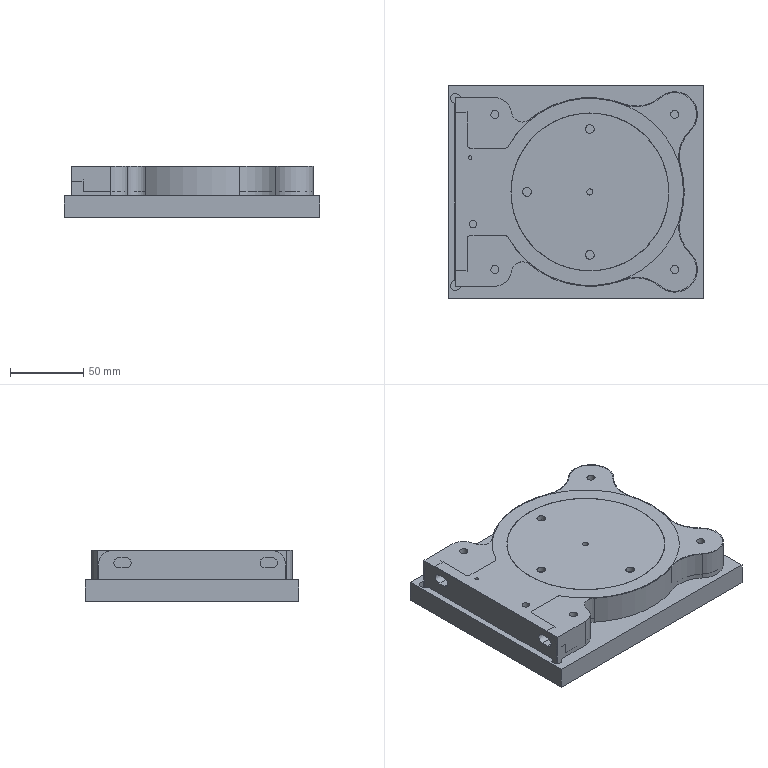NC program | NX | posted with a generic post | part box 175 x 146 x 35 mm
Lines 1 to 998 of 35144:
N10 G17 G21 G94 G90
(正面_COPY , TOOL : D10)
N12 T02 M6
N14 G54
N16 G17 G0 G90 X95.5 Y-68.762 S8000 M3
N18 G43 Z20. H2
N20 Z0.15
N22 G94 G1 X90.5 F2000.
N24 X-90.5
N26 Y-61.524
N28 X90.5
N30 Y-54.286
N32 X-90.5
N34 Y-47.048
N36 X90.5
N38 Y-39.81
N40 X-90.5
N42 Y-32.571
N44 X90.5
N46 Y-25.333
N48 X-90.5
N50 Y-18.095
N52 X90.5
N54 Y-10.857
N56 X-90.5
N58 Y-3.619
N60 X90.5
N62 Y3.619
N64 X-90.5
N66 Y10.857
N68 X90.5
N70 Y18.095
N72 X-90.5
N74 Y25.333
N76 X90.5
N78 Y32.571
N80 X-90.5
N82 Y39.81
N84 X90.5
N86 Y47.048
N88 X-90.5
N90 Y54.286
N92 X90.5
N94 Y61.524
N96 X-90.5
N98 Y68.762
N100 X90.5
N102 X95.5
N104 G0 Z20.
(跟随部件_COPY_2 , TOOL : D10)
N106 G1 X99.568 Y27.523 F15000.
N108 Z-1.4
N110 Z-1.9 F4000.
N112 G3 X92.497 Y27.582 R5.
N114 G2 X92.161 Y27.256 R35.65
N116 G3 X90.983 Y22.936 R4.35
N118 G2 X92.497 Y16.648 R84.65
N120 G3 X98.382 Y12.73 R5.
N122 G1 Z-1.4
N124 Z20. F15000.
N126 Y-12.73
N128 Z-1.4
N130 Z-1.9 F4000.
N132 G3 X92.497 Y-16.648 R5.
N134 G2 X90.983 Y-22.936 R84.65
N136 G3 X92.161 Y-27.256 R4.35
N138 G2 X92.497 Y-27.582 R35.65
N140 G1 Y-40.054
N142 G3 X86.973 Y-32.672 R28.15
N144 G2 X83.764 Y-20.904 R11.85
N146 G3 X83.764 Y20.904 R77.15
N148 G2 X86.973 Y32.672 R11.85
N150 G3 X92.497 Y40.054 R28.15
N152 G2 X99.236 Y42.195 R5.
N154 G1 Z-1.4
N156 Z20. F15000.
N158 X-36.967 Y85.011
N160 Z-1.4
N162 Z-1.9 F4000.
N164 G3 X-36.085 Y77.996 R5.
N166 G2 X-31.749 Y73.92 R31.65
N168 X-23.399 Y77.996 R84.65
N170 G3 X-20.735 Y84.546 R5.
N172 G1 Z-1.4
N174 Z20. F15000.
N176 X56.692 Y84.735
N178 Z-1.4
N180 Z-1.9 F4000.
N182 G2 X54.552 Y77.996 R5.
N184 G3 X49.005 Y74.222 R28.15
N186 G2 X36.997 Y72.084 R11.85
N188 G3 X-33.894 Y63.789 R77.15
N190 X-55.5 Y77.15 R24.15
N192 G1 X-82.502
N194 G3 X-92.497 Y72.543 R13.15
N196 G2 X-99.546 Y71.991 R5.
N198 G1 Z-1.4
N200 Z20. F15000.
N202 X-20.735 Y-84.546
N204 Z-1.4
N206 Z-1.9 F4000.
N208 G3 X-23.399 Y-77.996 R5.
N210 G2 X-31.749 Y-73.92 R84.65
N212 X-36.085 Y-77.996 R31.65
N214 G3 X-36.967 Y-85.011 R5.
N216 G1 Z-1.4
N218 Z20. F15000.
N220 X-99.546 Y-71.991
N222 Z-1.4
N224 Z-1.9 F4000.
N226 G2 X-92.497 Y-72.543 R5.
N228 G3 X-82.5 Y-77.15 R13.15
N230 G1 X-55.5
N232 G3 X-33.894 Y-63.789 R24.15
N234 X36.997 Y-72.084 R77.15
N236 G2 X49.005 Y-74.222 R11.85
N238 G3 X54.552 Y-77.996 R28.15
N240 G2 X56.692 Y-84.735 R5.
N242 G1 Z-1.4
N244 Z20. F15000.
N246 X78.308
N248 Z-1.4
N250 Z-1.9 F4000.
N252 G2 X80.448 Y-77.996 R5.
N254 G3 X92.497 Y-65.946 R28.15
N256 G2 X99.236 Y-63.805 R5.
N258 G1 Z-1.4
N260 Z20. F15000.
N262 Y63.805
N264 Z-1.4
N266 Z-1.9 F4000.
N268 G2 X92.497 Y65.946 R5.
N270 G3 X80.448 Y77.996 R28.15
N272 G1 X76.998 Y71.336
N274 G2 X81.785 Y38.088 R20.65
N276 G3 X76.545 Y18.872 R19.35
N278 G2 X76.545 Y-18.872 R69.65
N280 G3 X81.785 Y-38.088 R19.35
N282 G2 X53.933 Y-68.568 R20.65
N284 G3 X34.324 Y-65.076 R19.35
N286 G2 X-35.131 Y-53.472 R69.65
N288 G3 X-38.97 Y-54.994 R2.35
N290 G2 X-55.5 Y-69.65 R16.65
N292 G1 X-82.5
N294 G2 X-88.15 Y-64. R5.65
N296 G1 Y64.
N298 G2 X-82.5 Y69.65 R5.65
N300 G1 X-55.5
N302 G2 X-38.97 Y54.994 R16.65
N304 G3 X-35.131 Y53.472 R2.35
N306 G2 X34.324 Y65.076 R69.65
N308 G3 X53.933 Y68.568 R19.35
N310 G2 X76.998 Y71.336 R20.65
N312 G3 X83.738 Y73.476 R5.
N314 G1 Z-1.4
N316 Z20. F15000.
N318 X99.568 Y27.523
N320 Z-2.9
N322 Z-3.4 F4000.
N324 G3 X92.497 Y27.582 R5.
N326 G2 X92.161 Y27.256 R35.65
N328 G3 X90.983 Y22.936 R4.35
N330 G2 X92.497 Y16.648 R84.65
N332 G3 X98.383 Y12.728 R5.
N334 G1 Z-2.9
N336 Z20. F15000.
N338 Y-12.728
N340 Z-2.9
N342 Z-3.4 F4000.
N344 G3 X92.497 Y-16.648 R5.
N346 G2 X90.983 Y-22.936 R84.65
N348 G3 X92.161 Y-27.256 R4.35
N350 G2 X92.497 Y-27.582 R35.65
N352 G1 Y-40.055
N354 G3 X86.973 Y-32.672 R28.15
N356 G2 X83.764 Y-20.904 R11.85
N358 G3 X83.764 Y20.904 R77.15
N360 G2 X86.973 Y32.672 R11.85
N362 G3 X92.497 Y40.055 R28.15
N364 G2 X99.236 Y42.195 R5.
N366 G1 Z-2.9
N368 Z20. F15000.
N370 X-36.967 Y85.012
N372 Z-2.9
N374 Z-3.4 F4000.
N376 G3 X-36.085 Y77.996 R5.
N378 G2 X-31.749 Y73.92 R31.65
N380 X-23.398 Y77.996 R84.65
N382 G3 X-20.734 Y84.546 R5.
N384 G1 Z-2.9
N386 Z20. F15000.
N388 X56.693 Y84.735
N390 Z-2.9
N392 Z-3.4 F4000.
N394 G2 X54.553 Y77.996 R5.
N396 G3 X49.005 Y74.222 R28.15
N398 G2 X36.997 Y72.084 R11.85
N400 G3 X-33.894 Y63.789 R77.15
N402 X-55.5 Y77.15 R24.15
N404 G1 X-82.502
N406 G3 X-92.497 Y72.543 R13.15
N408 G2 X-99.546 Y71.99 R5.
N410 G1 Z-2.9
N412 Z20. F15000.
N414 X-20.734 Y-84.546
N416 Z-2.9
N418 Z-3.4 F4000.
N420 G3 X-23.398 Y-77.996 R5.
N422 G2 X-31.749 Y-73.92 R84.65
N424 X-36.085 Y-77.996 R31.65
N426 G3 X-36.967 Y-85.012 R5.
N428 G1 Z-2.9
N430 Z20. F15000.
N432 X-99.546 Y-71.99
N434 Z-2.9
N436 Z-3.4 F4000.
N438 G2 X-92.497 Y-72.543 R5.
N440 G3 X-82.5 Y-77.15 R13.15
N442 G1 X-55.5
N444 G3 X-33.894 Y-63.789 R24.15
N446 X36.997 Y-72.084 R77.15
N448 G2 X49.005 Y-74.222 R11.85
N450 G3 X54.553 Y-77.996 R28.15
N452 G2 X56.693 Y-84.735 R5.
N454 G1 Z-2.9
N456 Z20. F15000.
N458 X78.307
N460 Z-2.9
N462 Z-3.4 F4000.
N464 G2 X80.447 Y-77.996 R5.
N466 G3 X92.497 Y-65.945 R28.15
N468 G2 X99.236 Y-63.805 R5.
N470 G1 Z-2.9
N472 Z20. F15000.
N474 Y63.805
N476 Z-2.9
N478 Z-3.4 F4000.
N480 G2 X92.497 Y65.945 R5.
N482 G3 X80.447 Y77.996 R28.15
N484 G1 X76.998 Y71.336
N486 G2 X81.785 Y38.088 R20.65
N488 G3 X76.545 Y18.872 R19.35
N490 G2 X76.545 Y-18.872 R69.65
N492 G3 X81.785 Y-38.088 R19.35
N494 G2 X53.933 Y-68.568 R20.65
N496 G3 X34.324 Y-65.076 R19.35
N498 G2 X-35.131 Y-53.472 R69.65
N500 G3 X-38.97 Y-54.994 R2.35
N502 G2 X-55.5 Y-69.65 R16.65
N504 G1 X-82.5
N506 G2 X-88.15 Y-64. R5.65
N508 G1 Y64.
N510 G2 X-82.5 Y69.65 R5.65
N512 G1 X-55.5
N514 G2 X-38.97 Y54.994 R16.65
N516 G3 X-35.131 Y53.472 R2.35
N518 G2 X34.324 Y65.076 R69.65
N520 G3 X53.933 Y68.568 R19.35
N522 G2 X76.998 Y71.336 R20.65
N524 G3 X83.737 Y73.476 R5.
N526 G1 Z-2.9
N528 Z20. F15000.
N530 X99.568 Y27.523
N532 Z-4.65
N534 Z-5.15 F4000.
N536 G3 X92.497 Y27.582 R5.
N538 G2 X92.161 Y27.256 R35.65
N540 G3 X90.983 Y22.936 R4.35
N542 G2 X92.497 Y16.646 R84.65
N544 G3 X98.383 Y12.727 R5.
N546 G1 Z-4.65
N548 Z20. F15000.
N550 Y-12.727
N552 Z-4.65
N554 Z-5.15 F4000.
N556 G3 X92.497 Y-16.646 R5.
N558 G2 X90.983 Y-22.936 R84.65
N560 G3 X92.161 Y-27.256 R4.35
N562 G2 X92.497 Y-27.582 R35.65
N564 G1 Y-40.055
N566 G3 X86.973 Y-32.672 R28.15
N568 G2 X83.764 Y-20.904 R11.85
N570 G3 X83.764 Y20.904 R77.15
N572 G2 X86.973 Y32.672 R11.85
N574 G3 X92.497 Y40.055 R28.15
N576 G2 X99.236 Y42.196 R5.
N578 G1 Z-4.65
N580 Z20. F15000.
N582 X-36.967 Y85.012
N584 Z-4.65
N586 Z-5.15 F4000.
N588 G3 X-36.086 Y77.996 R5.
N590 G2 X-31.749 Y73.92 R31.65
N592 X-23.397 Y77.996 R84.65
N594 G3 X-20.734 Y84.546 R5.
N596 G1 Z-4.65
N598 Z20. F15000.
N600 X56.693 Y84.735
N602 Z-4.65
N604 Z-5.15 F4000.
N606 G2 X54.553 Y77.996 R5.
N608 G3 X49.005 Y74.222 R28.15
N610 G2 X36.997 Y72.084 R11.85
N612 G3 X-33.894 Y63.789 R77.15
N614 X-55.5 Y77.15 R24.15
N616 G1 X-82.502
N618 G3 X-92.497 Y72.543 R13.15
N620 G2 X-99.547 Y71.99 R5.
N622 G1 Z-4.65
N624 Z20. F15000.
N626 X-20.734 Y-84.546
N628 Z-4.65
N630 Z-5.15 F4000.
N632 G3 X-23.397 Y-77.996 R5.
N634 G2 X-31.749 Y-73.92 R84.65
N636 X-36.086 Y-77.996 R31.65
N638 G3 X-36.967 Y-85.012 R5.
N640 G1 Z-4.65
N642 Z20. F15000.
N644 X-99.547 Y-71.99
N646 Z-4.65
N648 Z-5.15 F4000.
N650 G2 X-92.497 Y-72.543 R5.
N652 G3 X-82.5 Y-77.15 R13.15
N654 G1 X-55.5
N656 G3 X-33.894 Y-63.789 R24.15
N658 X36.997 Y-72.084 R77.15
N660 G2 X49.005 Y-74.222 R11.85
N662 G3 X54.553 Y-77.996 R28.15
N664 G2 X56.693 Y-84.735 R5.
N666 G1 Z-4.65
N668 Z20. F15000.
N670 X78.307
N672 Z-4.65
N674 Z-5.15 F4000.
N676 G2 X80.447 Y-77.996 R5.
N678 G3 X92.497 Y-65.945 R28.15
N680 G2 X99.236 Y-63.804 R5.
N682 G1 Z-4.65
N684 Z20. F15000.
N686 Y63.804
N688 Z-4.65
N690 Z-5.15 F4000.
N692 G2 X92.497 Y65.945 R5.
N694 G3 X80.447 Y77.996 R28.15
N696 G1 X76.997 Y71.336
N698 G2 X81.785 Y38.088 R20.65
N700 G3 X76.545 Y18.872 R19.35
N702 G2 X76.545 Y-18.872 R69.65
N704 G3 X81.785 Y-38.088 R19.35
N706 G2 X53.933 Y-68.568 R20.65
N708 G3 X34.324 Y-65.076 R19.35
N710 G2 X-35.131 Y-53.472 R69.65
N712 G3 X-38.97 Y-54.994 R2.35
N714 G2 X-55.5 Y-69.65 R16.65
N716 G1 X-82.5
N718 G2 X-88.15 Y-64. R5.65
N720 G1 Y64.
N722 G2 X-82.5 Y69.65 R5.65
N724 G1 X-55.5
N726 G2 X-38.97 Y54.994 R16.65
N728 G3 X-35.131 Y53.472 R2.35
N730 G2 X34.324 Y65.076 R69.65
N732 G3 X53.933 Y68.568 R19.35
N734 G2 X76.997 Y71.336 R20.65
N736 G3 X83.737 Y73.477 R5.
N738 G1 Z-4.65
N740 Z20. F15000.
N742 X99.568 Y27.523
N744 Z-6.4
N746 Z-6.9 F4000.
N748 G3 X92.497 Y27.582 R5.
N750 G2 X92.161 Y27.256 R35.65
N752 G3 X90.983 Y22.936 R4.35
N754 G2 X92.497 Y16.645 R84.65
N756 G3 X98.383 Y12.726 R5.
N758 G1 Z-6.4
N760 Z20. F15000.
N762 Y-12.726
N764 Z-6.4
N766 Z-6.9 F4000.
N768 G3 X92.497 Y-16.645 R5.
N770 G2 X90.983 Y-22.936 R84.65
N772 G3 X92.161 Y-27.256 R4.35
N774 G2 X92.497 Y-27.582 R35.65
N776 G1 Y-40.056
N778 G3 X86.973 Y-32.672 R28.15
N780 G2 X83.764 Y-20.904 R11.85
N782 G3 X83.764 Y20.904 R77.15
N784 G2 X86.973 Y32.672 R11.85
N786 G3 X92.497 Y40.056 R28.15
N788 G2 X99.237 Y42.197 R5.
N790 G1 Z-6.4
N792 Z20. F15000.
N794 X-36.968 Y85.012
N796 Z-6.4
N798 Z-6.9 F4000.
N800 G3 X-36.086 Y77.996 R5.
N802 G2 X-31.749 Y73.92 R31.65
N804 X-23.397 Y77.996 R84.65
N806 G3 X-20.733 Y84.546 R5.
N808 G1 Z-6.4
N810 Z20. F15000.
N812 X56.694 Y84.736
N814 Z-6.4
N816 Z-6.9 F4000.
N818 G2 X54.554 Y77.996 R5.
N820 G3 X49.005 Y74.222 R28.15
N822 G2 X36.997 Y72.084 R11.85
N824 G3 X-33.894 Y63.789 R77.15
N826 X-55.5 Y77.15 R24.15
N828 G1 X-82.502
N830 G3 X-92.497 Y72.543 R13.15
N832 G2 X-99.547 Y71.989 R5.
N834 G1 Z-6.4
N836 Z20. F15000.
N838 X-20.733 Y-84.546
N840 Z-6.4
N842 Z-6.9 F4000.
N844 G3 X-23.397 Y-77.996 R5.
N846 G2 X-31.749 Y-73.92 R84.65
N848 X-36.086 Y-77.996 R31.65
N850 G3 X-36.968 Y-85.012 R5.
N852 G1 Z-6.4
N854 Z20. F15000.
N856 X-99.547 Y-71.989
N858 Z-6.4
N860 Z-6.9 F4000.
N862 G2 X-92.497 Y-72.543 R5.
N864 G3 X-82.5 Y-77.15 R13.15
N866 G1 X-55.5
N868 G3 X-33.894 Y-63.789 R24.15
N870 X36.997 Y-72.084 R77.15
N872 G2 X49.005 Y-74.222 R11.85
N874 G3 X54.554 Y-77.996 R28.15
N876 G2 X56.694 Y-84.736 R5.
N878 G1 Z-6.4
N880 Z20. F15000.
N882 X78.306
N884 Z-6.4
N886 Z-6.9 F4000.
N888 G2 X80.446 Y-77.996 R5.
N890 G3 X92.497 Y-65.944 R28.15
N892 G2 X99.237 Y-63.803 R5.
N894 G1 Z-6.4
N896 Z20. F15000.
N898 Y63.803
N900 Z-6.4
N902 Z-6.9 F4000.
N904 G2 X92.497 Y65.944 R5.
N906 G3 X80.446 Y77.996 R28.15
N908 G1 X76.997 Y71.337
N910 G2 X81.785 Y38.088 R20.65
N912 G3 X76.545 Y18.872 R19.35
N914 G2 X76.545 Y-18.872 R69.65
N916 G3 X81.785 Y-38.088 R19.35
N918 G2 X53.933 Y-68.568 R20.65
N920 G3 X34.324 Y-65.076 R19.35
N922 G2 X-35.131 Y-53.472 R69.65
N924 G3 X-38.97 Y-54.994 R2.35
N926 G2 X-55.5 Y-69.65 R16.65
N928 G1 X-82.5
N930 G2 X-88.15 Y-64. R5.65
N932 G1 Y64.
N934 G2 X-82.5 Y69.65 R5.65
N936 G1 X-55.5
N938 G2 X-38.97 Y54.994 R16.65
N940 G3 X-35.131 Y53.472 R2.35
N942 G2 X34.324 Y65.076 R69.65
N944 G3 X53.933 Y68.568 R19.35
N946 G2 X76.997 Y71.337 R20.65
N948 G3 X83.736 Y73.477 R5.
N950 G1 Z-6.4
N952 Z20. F15000.
N954 X99.568 Y27.524
N956 Z-7.9
N958 Z-8.4 F4000.
N960 G3 X92.498 Y27.583 R5.
N962 G2 X92.161 Y27.256 R35.65
N964 G3 X90.983 Y22.936 R4.35
N966 G2 X92.498 Y16.644 R84.65
N968 G3 X98.383 Y12.725 R5.
N970 G1 Z-7.9
N972 Z20. F15000.
N974 Y-12.725
N976 Z-7.9
N978 Z-8.4 F4000.
N980 G3 X92.498 Y-16.644 R5.
N982 G2 X90.983 Y-22.936 R84.65
N984 G3 X92.161 Y-27.256 R4.35
N986 G2 X92.498 Y-27.583 R35.65
N988 G1 Y-40.056
N990 G3 X86.973 Y-32.672 R28.15
N992 G2 X83.764 Y-20.904 R11.85
N994 G3 X83.764 Y20.904 R77.15
N996 G2 X86.973 Y32.672 R11.85
N998 G3 X92.498 Y40.056 R28.15
N1000 G2 X99.237 Y42.197 R5.
N1002 G1 Z-7.9
N1004 Z20. F15000.
N1006 X-36.968 Y85.012
N1008 Z-7.9
N1010 Z-8.4 F4000.
N1012 G3 X-36.086 Y77.997 R5.
N1014 G2 X-31.749 Y73.92 R31.65
N1016 X-23.396 Y77.997 R84.65
N1018 G3 X-20.732 Y84.547 R5.
N1020 G1 Z-7.9
N1022 Z20. F15000.
N1024 X56.695 Y84.736
N1026 Z-7.9
N1028 Z-8.4 F4000.
N1030 G2 X54.554 Y77.997 R5.
N1032 G3 X49.005 Y74.222 R28.15
N1034 G2 X36.997 Y72.084 R11.85
N1036 G3 X-33.894 Y63.789 R77.15
N1038 X-55.5 Y77.15 R24.15
N1040 G1 X-82.502
N1042 G3 X-92.498 Y72.542 R13.15
N1044 G2 X-99.547 Y71.989 R5.
N1046 G1 Z-7.9
N1048 Z20. F15000.
N1050 X-20.732 Y-84.547
N1052 Z-7.9
N1054 Z-8.4 F4000.
N1056 G3 X-23.396 Y-77.997 R5.
N1058 G2 X-31.749 Y-73.92 R84.65
N1060 X-36.086 Y-77.997 R31.65
N1062 G3 X-36.968 Y-85.012 R5.
N1064 G1 Z-7.9
N1066 Z20. F15000.
N1068 X-99.547 Y-71.989
N1070 Z-7.9
N1072 Z-8.4 F4000.
N1074 G2 X-92.498 Y-72.542 R5.
N1076 G3 X-82.5 Y-77.15 R13.15
N1078 G1 X-55.5
N1080 G3 X-33.894 Y-63.789 R24.15
N1082 X36.997 Y-72.084 R77.15
N1084 G2 X49.005 Y-74.222 R11.85
N1086 G3 X54.554 Y-77.997 R28.15
N1088 G2 X56.695 Y-84.736 R5.
N1090 G1 Z-7.9
N1092 Z20. F15000.
N1094 X78.305
N1096 Z-7.9
N1098 Z-8.4 F4000.
N1100 G2 X80.446 Y-77.997 R5.
N1102 G3 X92.498 Y-65.944 R28.15
N1104 G2 X99.237 Y-63.803 R5.
N1106 G1 Z-7.9
N1108 Z20. F15000.
N1110 Y63.803
N1112 Z-7.9
N1114 Z-8.4 F4000.
N1116 G2 X92.498 Y65.944 R5.
N1118 G3 X80.446 Y77.997 R28.15
N1120 G1 X76.997 Y71.337
N1122 G2 X81.785 Y38.088 R20.65
N1124 G3 X76.545 Y18.872 R19.35
N1126 G2 X76.545 Y-18.872 R69.65
N1128 G3 X81.785 Y-38.088 R19.35
N1130 G2 X53.933 Y-68.568 R20.65
N1132 G3 X34.324 Y-65.076 R19.35
N1134 G2 X-35.131 Y-53.472 R69.65
N1136 G3 X-38.97 Y-54.994 R2.35
N1138 G2 X-55.5 Y-69.65 R16.65
N1140 G1 X-82.5
N1142 G2 X-88.15 Y-64. R5.65
N1144 G1 Y64.
N1146 G2 X-82.5 Y69.65 R5.65
N1148 G1 X-55.5
N1150 G2 X-38.97 Y54.994 R16.65
N1152 G3 X-35.131 Y53.472 R2.35
N1154 G2 X34.324 Y65.076 R69.65
N1156 G3 X53.933 Y68.568 R19.35
N1158 G2 X76.997 Y71.337 R20.65
N1160 G3 X83.736 Y73.477 R5.
N1162 G1 Z-7.9
N1164 Z20. F15000.
N1166 X99.569 Y27.524
N1168 Z-9.4
N1170 Z-9.9 F4000.
N1172 G3 X92.498 Y27.583 R5.
N1174 G2 X92.161 Y27.256 R35.65
N1176 G3 X90.983 Y22.936 R4.35
N1178 G2 X92.498 Y16.643 R84.65
N1180 G3 X98.383 Y12.724 R5.
N1182 G1 Z-9.4
N1184 Z20. F15000.
N1186 Y-12.724
N1188 Z-9.4
N1190 Z-9.9 F4000.
N1192 G3 X92.498 Y-16.643 R5.
N1194 G2 X90.983 Y-22.936 R84.65
N1196 G3 X92.161 Y-27.256 R4.35
N1198 G2 X92.498 Y-27.583 R35.65
N1200 G1 Y-40.056
N1202 G3 X86.973 Y-32.672 R28.15
N1204 G2 X83.764 Y-20.904 R11.85
N1206 G3 X83.764 Y20.904 R77.15
N1208 G2 X86.973 Y32.672 R11.85
N1210 G3 X92.498 Y40.056 R28.15
N1212 G2 X99.237 Y42.198 R5.
N1214 G1 Z-9.4
N1216 Z20. F15000.
N1218 X-36.969 Y85.013
N1220 Z-9.4
N1222 Z-9.9 F4000.
N1224 G3 X-36.087 Y77.997 R5.
N1226 G2 X-31.749 Y73.92 R31.65
N1228 X-23.396 Y77.997 R84.65
N1230 G3 X-20.732 Y84.547 R5.
N1232 G1 Z-9.4
N1234 Z20. F15000.
N1236 X56.695 Y84.736
N1238 Z-9.4
N1240 Z-9.9 F4000.
N1242 G2 X54.555 Y77.997 R5.
N1244 G3 X49.005 Y74.222 R28.15
N1246 G2 X36.997 Y72.084 R11.85
N1248 G3 X-33.894 Y63.789 R77.15
N1250 X-55.5 Y77.15 R24.15
N1252 G1 X-82.502
N1254 G3 X-92.498 Y72.542 R13.15
N1256 G2 X-99.547 Y71.989 R5.
N1258 G1 Z-9.4
N1260 Z20. F15000.
N1262 X-20.732 Y-84.547
N1264 Z-9.4
N1266 Z-9.9 F4000.
N1268 G3 X-23.396 Y-77.997 R5.
N1270 G2 X-31.749 Y-73.92 R84.65
N1272 X-36.087 Y-77.997 R31.65
N1274 G3 X-36.969 Y-85.013 R5.
N1276 G1 Z-9.4
N1278 Z20. F15000.
N1280 X-99.547 Y-71.989
N1282 Z-9.4
N1284 Z-9.9 F4000.
N1286 G2 X-92.498 Y-72.542 R5.
N1288 G3 X-82.5 Y-77.15 R13.15
N1290 G1 X-55.5
N1292 G3 X-33.894 Y-63.789 R24.15
N1294 X36.997 Y-72.084 R77.15
N1296 G2 X49.005 Y-74.222 R11.85
N1298 G3 X54.555 Y-77.997 R28.15
N1300 G2 X56.695 Y-84.736 R5.
N1302 G1 Z-9.4
N1304 Z20. F15000.
N1306 X78.305
N1308 Z-9.4
N1310 Z-9.9 F4000.
N1312 G2 X80.445 Y-77.997 R5.
N1314 G3 X92.498 Y-65.944 R28.15
N1316 G2 X99.237 Y-63.802 R5.
N1318 G1 Z-9.4
N1320 Z20. F15000.
N1322 Y63.802
N1324 Z-9.4
N1326 Z-9.9 F4000.
N1328 G2 X92.498 Y65.944 R5.
N1330 G3 X80.445 Y77.997 R28.15
N1332 G1 X76.996 Y71.337
N1334 G2 X81.785 Y38.088 R20.65
N1336 G3 X76.545 Y18.872 R19.35
N1338 G2 X76.545 Y-18.872 R69.65
N1340 G3 X81.785 Y-38.088 R19.35
N1342 G2 X53.933 Y-68.568 R20.65
N1344 G3 X34.324 Y-65.076 R19.35
N1346 G2 X-35.131 Y-53.472 R69.65
N1348 G3 X-38.97 Y-54.994 R2.35
N1350 G2 X-55.5 Y-69.65 R16.65
N1352 G1 X-82.5
N1354 G2 X-88.15 Y-64. R5.65
N1356 G1 Y64.
N1358 G2 X-82.5 Y69.65 R5.65
N1360 G1 X-55.5
N1362 G2 X-38.97 Y54.994 R16.65
N1364 G3 X-35.131 Y53.472 R2.35
N1366 G2 X34.324 Y65.076 R69.65
N1368 G3 X53.933 Y68.568 R19.35
N1370 G2 X76.996 Y71.337 R20.65
N1372 G3 X83.736 Y73.478 R5.
N1374 G1 Z-9.4
N1376 Z20. F15000.
N1378 X99.569 Y27.524
N1380 Z-11.9
N1382 Z-12.4 F4000.
N1384 G3 X92.498 Y27.583 R5.
N1386 G2 X92.161 Y27.256 R35.65
N1388 G3 X90.983 Y22.936 R4.35
N1390 G2 X92.498 Y16.642 R84.65
N1392 G3 X98.383 Y12.722 R5.
N1394 G1 Z-11.9
N1396 Z20. F15000.
N1398 Y-12.722
N1400 Z-11.9
N1402 Z-12.4 F4000.
N1404 G3 X92.498 Y-16.642 R5.
N1406 G2 X90.983 Y-22.936 R84.65
N1408 G3 X92.161 Y-27.256 R4.35
N1410 G2 X92.498 Y-27.583 R35.65
N1412 G1 Y-40.057
N1414 G3 X86.973 Y-32.672 R28.15
N1416 G2 X83.764 Y-20.904 R11.85
N1418 G3 X83.764 Y20.904 R77.15
N1420 G2 X86.973 Y32.672 R11.85
N1422 G3 X92.498 Y40.057 R28.15
N1424 G2 X99.237 Y42.198 R5.
N1426 G1 Z-11.9
N1428 Z20. F15000.
N1430 X-36.969 Y85.013
N1432 Z-11.9
N1434 Z-12.4 F4000.
N1436 G3 X-36.087 Y77.997 R5.
N1438 G2 X-31.749 Y73.92 R31.65
N1440 X-23.395 Y77.997 R84.65
N1442 G3 X-20.731 Y84.547 R5.
N1444 G1 Z-11.9
N1446 Z20. F15000.
N1448 X56.696 Y84.736
N1450 Z-11.9
N1452 Z-12.4 F4000.
N1454 G2 X54.555 Y77.997 R5.
N1456 G3 X49.005 Y74.222 R28.15
N1458 G2 X36.997 Y72.084 R11.85
N1460 G3 X-33.894 Y63.789 R77.15
N1462 X-55.5 Y77.15 R24.15
N1464 G1 X-82.502
N1466 G3 X-92.498 Y72.542 R13.15
N1468 G2 X-99.547 Y71.988 R5.
N1470 G1 Z-11.9
N1472 Z20. F15000.
N1474 X-20.731 Y-84.547
N1476 Z-11.9
N1478 Z-12.4 F4000.
N1480 G3 X-23.395 Y-77.997 R5.
N1482 G2 X-31.749 Y-73.92 R84.65
N1484 X-36.087 Y-77.997 R31.65
N1486 G3 X-36.969 Y-85.013 R5.
N1488 G1 Z-11.9
N1490 Z20. F15000.
N1492 X-99.547 Y-71.988
N1494 Z-11.9
N1496 Z-12.4 F4000.
N1498 G2 X-92.498 Y-72.542 R5.
N1500 G3 X-82.5 Y-77.15 R13.15
N1502 G1 X-55.5
N1504 G3 X-33.894 Y-63.789 R24.15
N1506 X36.997 Y-72.084 R77.15
N1508 G2 X49.005 Y-74.222 R11.85
N1510 G3 X54.555 Y-77.997 R28.15
N1512 G2 X56.696 Y-84.736 R5.
N1514 G1 Z-11.9
N1516 Z20. F15000.
N1518 X78.304
N1520 Z-11.9
N1522 Z-12.4 F4000.
N1524 G2 X80.445 Y-77.997 R5.
N1526 G3 X92.498 Y-65.943 R28.15
N1528 G2 X99.237 Y-63.802 R5.
N1530 G1 Z-11.9
N1532 Z20. F15000.
N1534 Y63.802
N1536 Z-11.9
N1538 Z-12.4 F4000.
N1540 G2 X92.498 Y65.943 R5.
N1542 G3 X80.445 Y77.997 R28.15
N1544 G1 X76.996 Y71.337
N1546 G2 X81.785 Y38.088 R20.65
N1548 G3 X76.545 Y18.872 R19.35
N1550 G2 X76.545 Y-18.872 R69.65
N1552 G3 X81.785 Y-38.088 R19.35
N1554 G2 X53.933 Y-68.568 R20.65
N1556 G3 X34.324 Y-65.076 R19.35
N1558 G2 X-35.131 Y-53.472 R69.65
N1560 G3 X-38.97 Y-54.994 R2.35
N1562 G2 X-55.5 Y-69.65 R16.65
N1564 G1 X-82.5
N1566 G2 X-88.15 Y-64. R5.65
N1568 G1 Y64.
N1570 G2 X-82.5 Y69.65 R5.65
N1572 G1 X-55.5
N1574 G2 X-38.97 Y54.994 R16.65
N1576 G3 X-35.131 Y53.472 R2.35
N1578 G2 X34.324 Y65.076 R69.65
N1580 G3 X53.933 Y68.568 R19.35
N1582 G2 X76.996 Y71.337 R20.65
N1584 G3 X83.735 Y73.478 R5.
N1586 G1 Z-11.9
N1588 Z20. F15000.
N1590 X99.569 Y27.525
N1592 Z-14.4
N1594 Z-14.9 F4000.
N1596 G3 X92.498 Y27.583 R5.
N1598 G2 X92.161 Y27.256 R35.65
N1600 G3 X90.983 Y22.936 R4.35
N1602 G2 X92.498 Y16.64 R84.65
N1604 G3 X98.384 Y12.72 R5.
N1606 G1 Z-14.4
N1608 Z20. F15000.
N1610 Y-12.72
N1612 Z-14.4
N1614 Z-14.9 F4000.
N1616 G3 X92.498 Y-16.64 R5.
N1618 G2 X90.983 Y-22.936 R84.65
N1620 G3 X92.161 Y-27.256 R4.35
N1622 G2 X92.498 Y-27.583 R35.65
N1624 G1 Y-40.058
N1626 G3 X86.973 Y-32.672 R28.15
N1628 G2 X83.764 Y-20.904 R11.85
N1630 G3 X83.764 Y20.904 R77.15
N1632 G2 X86.973 Y32.672 R11.85
N1634 G3 X92.498 Y40.058 R28.15
N1636 G2 X99.237 Y42.199 R5.
N1638 G1 Z-14.4
N1640 Z20. F15000.
N1642 X-36.97 Y85.013
N1644 Z-14.4
N1646 Z-14.9 F4000.
N1648 G3 X-36.088 Y77.998 R5.
N1650 G2 X-31.749 Y73.92 R31.65
N1652 X-23.394 Y77.998 R84.65
N1654 G3 X-20.73 Y84.548 R5.
N1656 G1 Z-14.4
N1658 Z20. F15000.
N1660 X56.697 Y84.737
N1662 Z-14.4
N1664 Z-14.9 F4000.
N1666 G2 X54.556 Y77.998 R5.
N1668 G3 X49.005 Y74.222 R28.15
N1670 G2 X36.997 Y72.084 R11.85
N1672 G3 X-33.894 Y63.789 R77.15
N1674 X-55.5 Y77.15 R24.15
N1676 G1 X-82.502
N1678 G3 X-92.498 Y72.541 R13.15
N1680 G2 X-99.548 Y71.987 R5.
N1682 G1 Z-14.4
N1684 Z20. F15000.
N1686 X-20.73 Y-84.548
N1688 Z-14.4
N1690 Z-14.9 F4000.
N1692 G3 X-23.394 Y-77.998 R5.
N1694 G2 X-31.749 Y-73.92 R84.65
N1696 X-36.088 Y-77.998 R31.65
N1698 G3 X-36.97 Y-85.013 R5.
N1700 G1 Z-14.4
N1702 Z20. F15000.
N1704 X-99.548 Y-71.987
N1706 Z-14.4
N1708 Z-14.9 F4000.
N1710 G2 X-92.498 Y-72.541 R5.
N1712 G3 X-82.5 Y-77.15 R13.15
N1714 G1 X-55.5
N1716 G3 X-33.894 Y-63.789 R24.15
N1718 X36.997 Y-72.084 R77.15
N1720 G2 X49.005 Y-74.222 R11.85
N1722 G3 X54.556 Y-77.998 R28.15
N1724 G2 X56.697 Y-84.737 R5.
N1726 G1 Z-14.4
N1728 Z20. F15000.
N1730 X78.303
N1732 Z-14.4
N1734 Z-14.9 F4000.
N1736 G2 X80.444 Y-77.998 R5.
N1738 G3 X92.498 Y-65.942 R28.15
N1740 G2 X99.237 Y-63.801 R5.
N1742 G1 Z-14.4
N1744 Z20. F15000.
N1746 Y63.801
N1748 Z-14.4
N1750 Z-14.9 F4000.
N1752 G2 X92.498 Y65.942 R5.
N1754 G3 X80.444 Y77.998 R28.15
N1756 G1 X76.995 Y71.338
N1758 G2 X81.785 Y38.088 R20.65
N1760 G3 X76.545 Y18.872 R19.35
N1762 G2 X76.545 Y-18.872 R69.65
N1764 G3 X81.785 Y-38.088 R19.35
N1766 G2 X53.933 Y-68.568 R20.65
N1768 G3 X34.324 Y-65.076 R19.35
N1770 G2 X-35.131 Y-53.472 R69.65
N1772 G3 X-38.97 Y-54.994 R2.35
N1774 G2 X-55.5 Y-69.65 R16.65
N1776 G1 X-82.5
N1778 G2 X-88.15 Y-64. R5.65
N1780 G1 Y64.
N1782 G2 X-82.5 Y69.65 R5.65
N1784 G1 X-55.5
N1786 G2 X-38.97 Y54.994 R16.65
N1788 G3 X-35.131 Y53.472 R2.35
N1790 G2 X34.324 Y65.076 R69.65
N1792 G3 X53.933 Y68.568 R19.35
N1794 G2 X76.995 Y71.338 R20.65
N1796 G3 X83.734 Y73.479 R5.
N1798 G1 Z-14.4
N1800 Z20. F15000.
N1802 X99.57 Y27.525
N1804 Z-16.9
N1806 Z-17.4 F4000.
N1808 G3 X92.499 Y27.584 R5.
N1810 G2 X92.161 Y27.256 R35.65
N1812 G3 X90.983 Y22.936 R4.35
N1814 G2 X92.499 Y16.638 R84.65
N1816 G3 X98.384 Y12.719 R5.
N1818 G1 Z-16.9
N1820 Z20. F15000.
N1822 Y-12.719
N1824 Z-16.9
N1826 Z-17.4 F4000.
N1828 G3 X92.499 Y-16.638 R5.
N1830 G2 X90.983 Y-22.936 R84.65
N1832 G3 X92.161 Y-27.256 R4.35
N1834 G2 X92.499 Y-27.584 R35.65
N1836 G1 Y-40.058
N1838 G3 X86.973 Y-32.672 R28.15
N1840 G2 X83.764 Y-20.904 R11.85
N1842 G3 X83.764 Y20.904 R77.15
N1844 G2 X86.973 Y32.672 R11.85
N1846 G3 X92.499 Y40.058 R28.15
N1848 G2 X99.238 Y42.2 R5.
N1850 G1 Z-16.9
N1852 Z20. F15000.
N1854 X-36.971 Y85.014
N1856 Z-16.9
N1858 Z-17.4 F4000.
N1860 G3 X-36.088 Y77.998 R5.
N1862 G2 X-31.749 Y73.92 R31.65
N1864 X-23.393 Y77.998 R84.65
N1866 G3 X-20.729 Y84.548 R5.
N1868 G1 Z-16.9
N1870 Z20. F15000.
N1872 X56.698 Y84.737
N1874 Z-16.9
N1876 Z-17.4 F4000.
N1878 G2 X54.557 Y77.998 R5.
N1880 G3 X49.005 Y74.222 R28.15
N1882 G2 X36.997 Y72.084 R11.85
N1884 G3 X-33.894 Y63.789 R77.15
N1886 X-55.5 Y77.15 R24.15
N1888 G1 X-82.5
N1890 G3 X-92.499 Y72.541 R13.15
N1892 G2 X-99.548 Y71.987 R5.
N1894 G1 Z-16.9
N1896 Z20. F15000.
N1898 X-20.729 Y-84.548
N1900 Z-16.9
N1902 Z-17.4 F4000.
N1904 G3 X-23.393 Y-77.998 R5.
N1906 G2 X-31.749 Y-73.92 R84.65
N1908 X-36.088 Y-77.998 R31.65
N1910 G3 X-36.971 Y-85.014 R5.
N1912 G1 Z-16.9
N1914 Z20. F15000.
N1916 X-99.548 Y-71.987
N1918 Z-16.9
N1920 Z-17.4 F4000.
N1922 G2 X-92.499 Y-72.541 R5.
N1924 G3 X-82.5 Y-77.15 R13.15
N1926 G1 X-55.5
N1928 G3 X-33.894 Y-63.789 R24.15
N1930 X36.997 Y-72.084 R77.15
N1932 G2 X49.005 Y-74.222 R11.85
N1934 G3 X54.557 Y-77.998 R28.15
N1936 G2 X56.698 Y-84.737 R5.
N1938 G1 Z-16.9
N1940 Z20. F15000.
N1942 X78.302
N1944 Z-16.9
N1946 Z-17.4 F4000.
N1948 G2 X80.443 Y-77.998 R5.
N1950 G3 X92.499 Y-65.942 R28.15
N1952 G2 X99.238 Y-63.8 R5.
N1954 G1 Z-16.9
N1956 Z20. F15000.
N1958 Y63.8
N1960 Z-16.9
N1962 Z-17.4 F4000.
N1964 G2 X92.499 Y65.942 R5.
N1966 G3 X80.443 Y77.998 R28.15
N1968 G1 X76.995 Y71.338
N1970 G2 X81.785 Y38.088 R20.65
N1972 G3 X76.545 Y18.872 R19.35
N1974 G2 X76.545 Y-18.872 R69.65
N1976 G3 X81.785 Y-38.088 R19.35
N1978 G2 X53.933 Y-68.568 R20.65
N1980 G3 X34.324 Y-65.076 R19.35
N1982 G2 X-35.131 Y-53.472 R69.65
N1984 G3 X-38.97 Y-54.994 R2.35
N1986 G2 X-55.5 Y-69.65 R16.65
N1988 G1 X-82.5